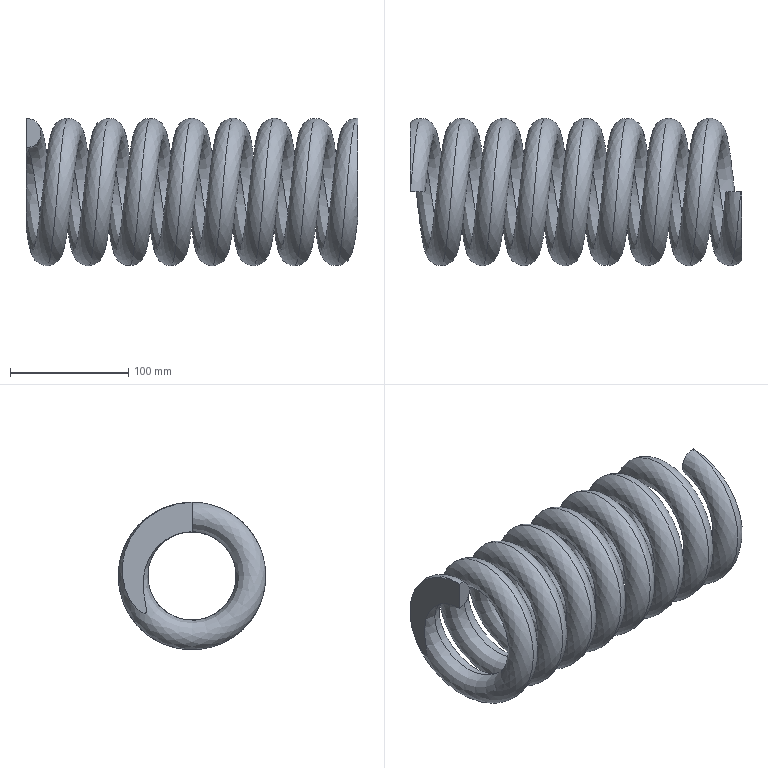Part | SolidWorks | features Helix 1, ICE 1, Sweep 1 | 1 solid | 6 faces | box 280.817 x 125 x 125 mm | volume 1207735 mm3 | plane 4 | spline 2